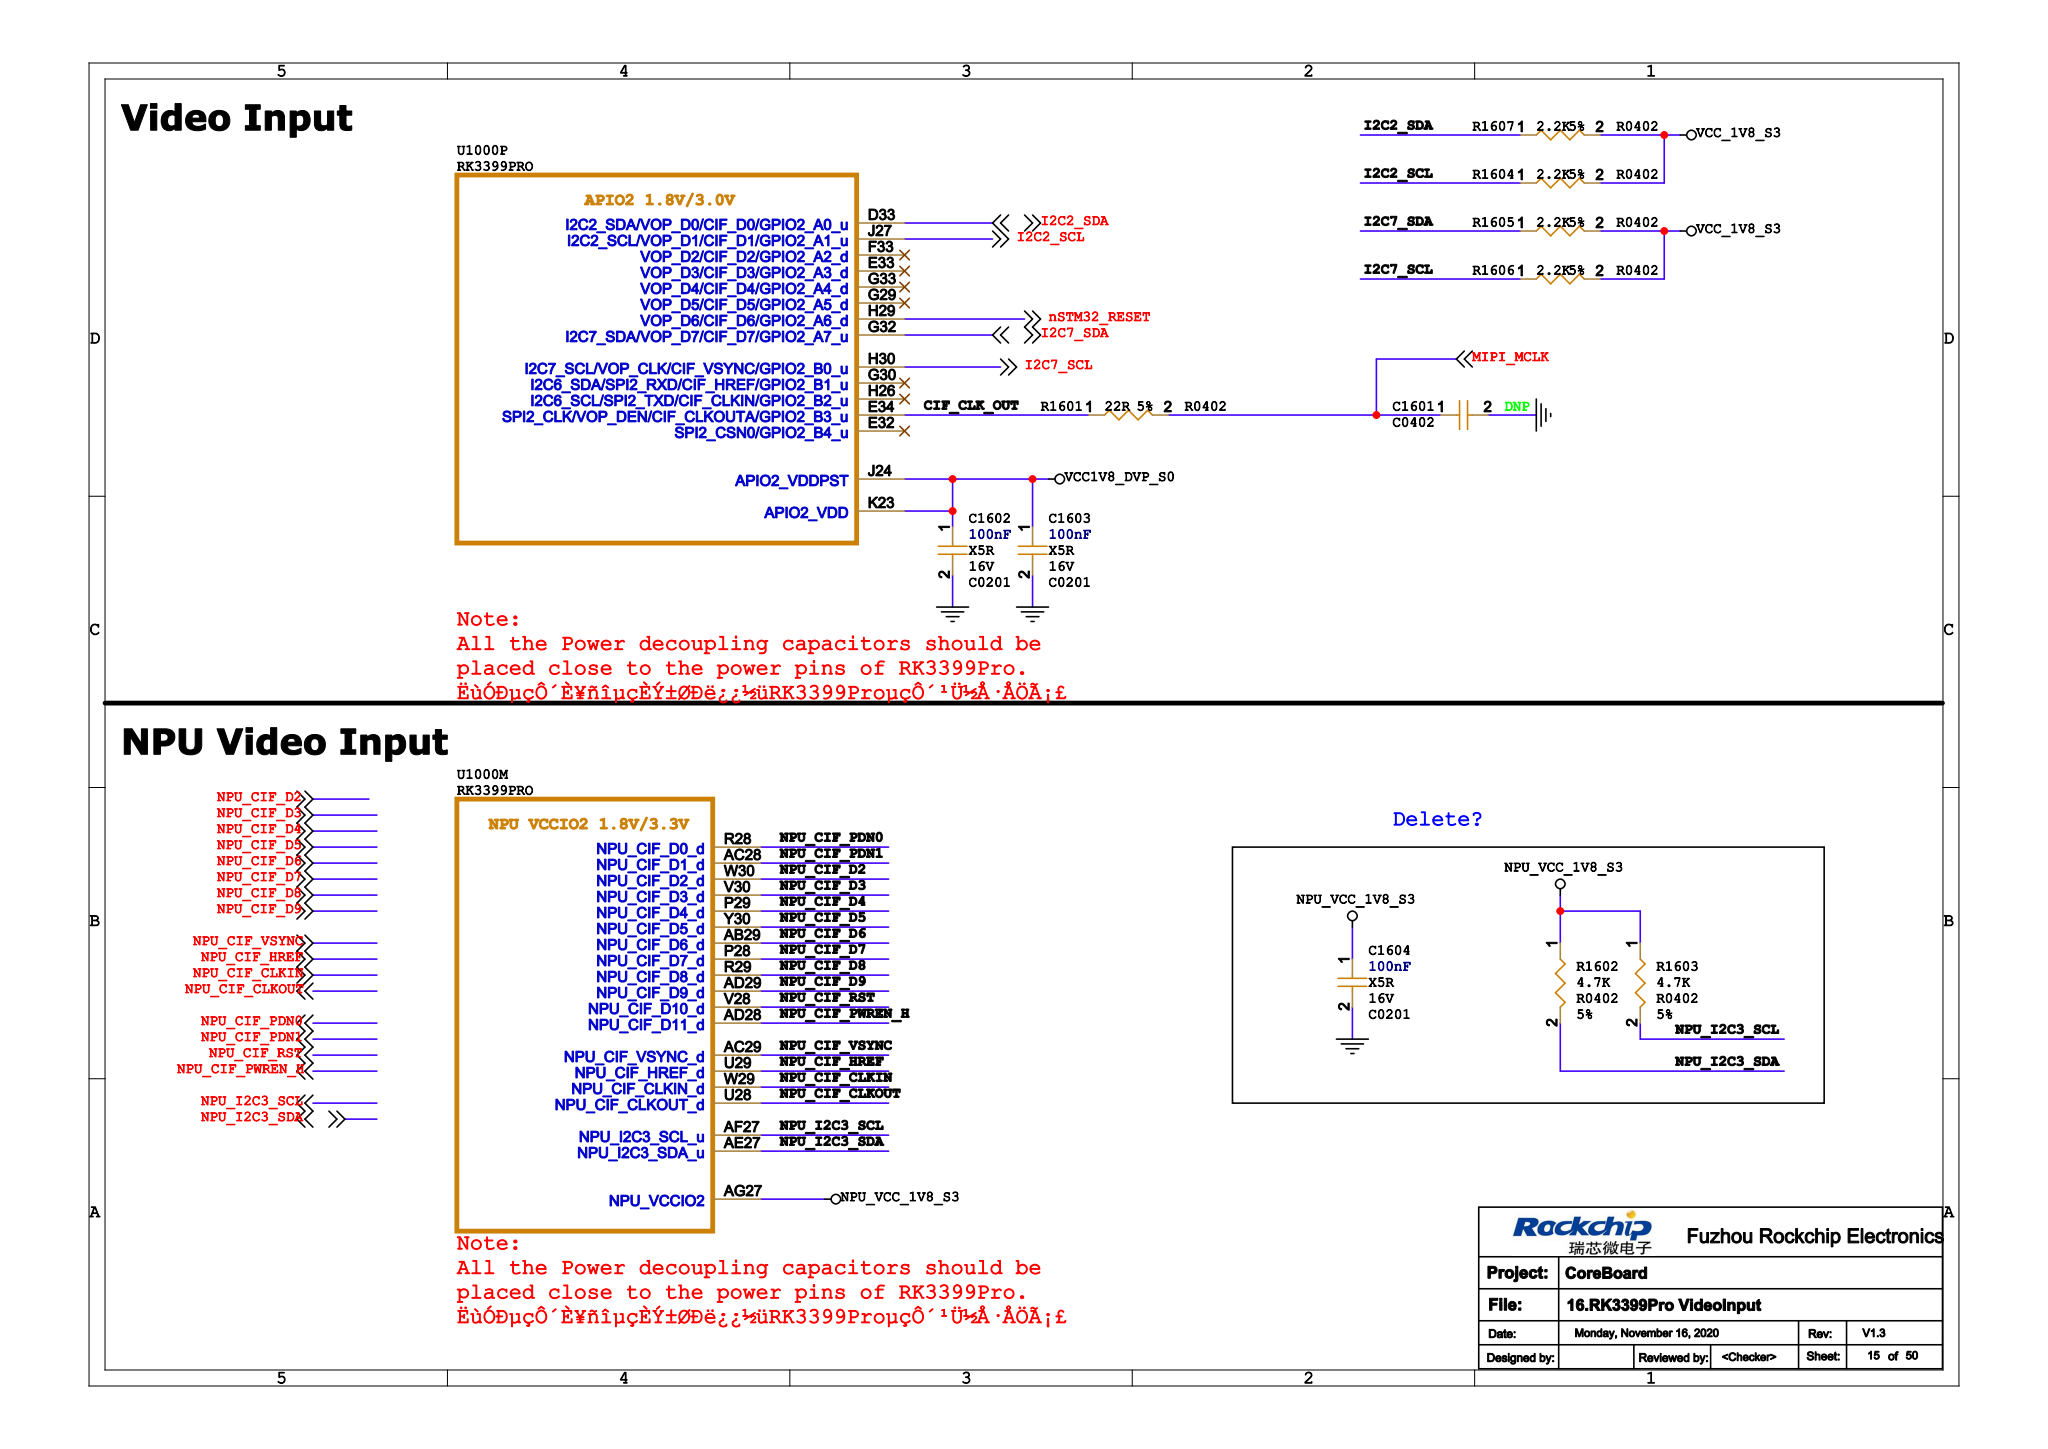Circuit board | Cadence Allegro | 749 parts | 717 nets | one sheet of the schematic
Parts on this sheet (reference | value | footprint):
C1601 | DNP | C0402
C1602 | 100nF | C0201
C1603 | 100nF | C0201
C1604 | 100nF | C0201
R1602 | 4.7K | R0402
R1603 | 4.7K | R0402
U1000 | RK3399PRO | BGA1372_27R00X27R00X2R19
Nets of these parts (net: part-pin ...):
GND: C1601-2 C1602-2 C1603-2 C1604-2
MIPI_MCLK: C1601-1
I2C2_SDA: U1000-D33
I2C2_SCL: U1000-J27
I2C7_SDA: U1000-G32
I2C7_SCL: U1000-H30
NPU_VCC_1V8_S3: C1604-1 R1602-1 R1603-1 U1000-AG27
NPU_I2C3_SDA: R1602-2 U1000-AE27
NPU_I2C3_SCL: R1603-2 U1000-AF27
VCC1V8_DVP_S0: C1602-1 C1603-1 U1000-J24 U1000-K23
CIF_CLK_OUT: U1000-E34
NPU_CIF_CLKIN: U1000-W29
NPU_CIF_CLKOUT: U1000-U28
NPU_CIF_D2: U1000-W30
NPU_CIF_D3: U1000-V30
NPU_CIF_D4: U1000-P29
NPU_CIF_D5: U1000-Y30
NPU_CIF_D6: U1000-AB29
NPU_CIF_D7: U1000-P28
NPU_CIF_D8: U1000-R29
NPU_CIF_D9: U1000-AD29
NPU_CIF_HREF: U1000-U29
NPU_CIF_VSYNC: U1000-AC29
NPU_CIF_PDN0: U1000-R28
NPU_CIF_RST: U1000-V28
NPU_CIF_PWREN_H: U1000-AD28
NPU_CIF_PDN1: U1000-AC28